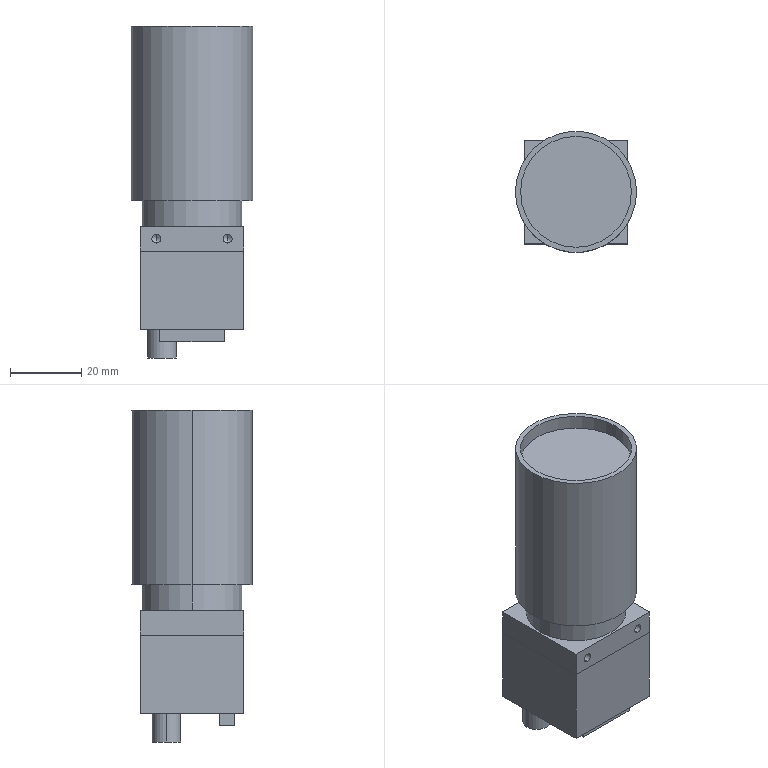Part | NX | features BREP 2 | 2 solids | 45 faces | box 34 x 34 x 93.2 mm | volume 70795 mm3 | plane 21 | cylinder 16 | cone 8 | commonest cylinder face diameters 2.5 x8 7.998 x2 28 x2 31.136 x2 34 x2
STEP:
#1=CARTESIAN_POINT('',(-12.39,7.192,-8.));
#2=VERTEX_POINT('',#1);
#3=CARTESIAN_POINT('',(-4.391,7.192,-8.));
#4=VERTEX_POINT('',#3);
#5=CARTESIAN_POINT('',(-8.39,7.192,-8.));
#6=DIRECTION('',(0.,0.,-1.));
#7=DIRECTION('',(-1.,0.,0.));
#8=AXIS2_PLACEMENT_3D('',#5,#6,#7);
#9=CIRCLE('',#8,3.999);
#10=EDGE_CURVE('',#2,#4,#9,.T.);
#11=ORIENTED_EDGE('',*,*,#10,.F.);
#12=CARTESIAN_POINT('',(-12.39,7.192,0.));
#13=VERTEX_POINT('',#12);
#14=CARTESIAN_POINT('',(-12.39,7.192,-8.));
#15=DIRECTION('',(0.,0.,1.));
#16=VECTOR('',#15,1000.);
#17=LINE('',#14,#16);
#18=EDGE_CURVE('',#13,#2,#17,.F.);
#19=ORIENTED_EDGE('',*,*,#18,.F.);
#20=CARTESIAN_POINT('',(-4.391,7.192,0.));
#21=VERTEX_POINT('',#20);
#22=CARTESIAN_POINT('',(-8.39,7.192,0.));
#23=DIRECTION('',(0.,0.,-1.));
#24=DIRECTION('',(-1.,0.,0.));
#25=AXIS2_PLACEMENT_3D('',#22,#23,#24);
#26=CIRCLE('',#25,3.999);
#27=EDGE_CURVE('',#13,#21,#26,.T.);
#28=ORIENTED_EDGE('',*,*,#27,.T.);
#29=CARTESIAN_POINT('',(-4.391,7.192,-8.));
#30=DIRECTION('',(0.,0.,1.));
#31=VECTOR('',#30,1000.);
#32=LINE('',#29,#31);
#33=EDGE_CURVE('',#21,#4,#32,.F.);
#34=ORIENTED_EDGE('',*,*,#33,.T.);
#35=EDGE_LOOP('',(#11,#19,#28,#34));
#36=FACE_BOUND('',#35,.T.);
#37=CARTESIAN_POINT('',(-8.39,7.192,-8.));
#38=DIRECTION('',(0.,0.,1.));
#39=DIRECTION('',(1.,0.,0.));
#40=AXIS2_PLACEMENT_3D('',#37,#38,#39);
#41=CYLINDRICAL_SURFACE('',#40,3.999);
#42=ADVANCED_FACE('',(#36),#41,.T.);
#43=CARTESIAN_POINT('',(14.5,-14.5,0.));
#44=VERTEX_POINT('',#43);
#45=CARTESIAN_POINT('',(14.5,14.5,0.));
#46=VERTEX_POINT('',#45);
#47=CARTESIAN_POINT('',(14.5,-14.5,0.));
#48=DIRECTION('',(0.,1.,0.));
#49=VECTOR('',#48,1000.);
#50=LINE('',#47,#49);
#51=EDGE_CURVE('',#44,#46,#50,.T.);
#52=ORIENTED_EDGE('',*,*,#51,.F.);
#53=CARTESIAN_POINT('',(-14.5,-14.5,0.));
#54=VERTEX_POINT('',#53);
#55=CARTESIAN_POINT('',(-14.5,-14.5,0.));
#56=DIRECTION('',(1.,0.,0.));
#57=VECTOR('',#56,1000.);
#58=LINE('',#55,#57);
#59=EDGE_CURVE('',#54,#44,#58,.T.);
#60=ORIENTED_EDGE('',*,*,#59,.F.);
#61=CARTESIAN_POINT('',(-14.5,14.5,0.));
#62=VERTEX_POINT('',#61);
#63=CARTESIAN_POINT('',(-14.5,-14.5,0.));
#64=DIRECTION('',(0.,-1.,0.));
#65=VECTOR('',#64,1000.);
#66=LINE('',#63,#65);
#67=EDGE_CURVE('',#62,#54,#66,.T.);
#68=ORIENTED_EDGE('',*,*,#67,.F.);
#69=CARTESIAN_POINT('',(-14.5,14.5,0.));
#70=DIRECTION('',(-1.,0.,0.));
#71=VECTOR('',#70,1000.);
#72=LINE('',#69,#71);
#73=EDGE_CURVE('',#46,#62,#72,.T.);
#74=ORIENTED_EDGE('',*,*,#73,.F.);
#75=EDGE_LOOP('',(#52,#60,#68,#74));
#76=FACE_BOUND('',#75,.T.);
#77=CARTESIAN_POINT('',(9.023,-12.03,0.));
#78=VERTEX_POINT('',#77);
#79=CARTESIAN_POINT('',(-9.023,-12.03,0.));
#80=VERTEX_POINT('',#79);
#81=CARTESIAN_POINT('',(-9.023,-12.03,0.));
#82=DIRECTION('',(-1.,0.,0.));
#83=VECTOR('',#82,1000.);
#84=LINE('',#81,#83);
#85=EDGE_CURVE('',#78,#80,#84,.T.);
#86=ORIENTED_EDGE('',*,*,#85,.F.);
#87=CARTESIAN_POINT('',(9.023,-7.6,0.));
#88=VERTEX_POINT('',#87);
#89=CARTESIAN_POINT('',(9.023,-12.03,0.));
#90=DIRECTION('',(0.,-1.,0.));
#91=VECTOR('',#90,1000.);
#92=LINE('',#89,#91);
#93=EDGE_CURVE('',#88,#78,#92,.T.);
#94=ORIENTED_EDGE('',*,*,#93,.F.);
#95=CARTESIAN_POINT('',(-9.023,-7.6,0.));
#96=VERTEX_POINT('',#95);
#97=CARTESIAN_POINT('',(-9.023,-7.6,0.));
#98=DIRECTION('',(1.,0.,0.));
#99=VECTOR('',#98,1000.);
#100=LINE('',#97,#99);
#101=EDGE_CURVE('',#96,#88,#100,.T.);
#102=ORIENTED_EDGE('',*,*,#101,.F.);
#103=CARTESIAN_POINT('',(-9.023,-12.03,0.));
#104=DIRECTION('',(0.,1.,0.));
#105=VECTOR('',#104,1000.);
#106=LINE('',#103,#105);
#107=EDGE_CURVE('',#80,#96,#106,.T.);
#108=ORIENTED_EDGE('',*,*,#107,.F.);
#109=EDGE_LOOP('',(#86,#94,#102,#108));
#110=FACE_BOUND('',#109,.T.);
#111=CARTESIAN_POINT('',(-8.39,7.192,0.));
#112=DIRECTION('',(0.,0.,-1.));
#113=DIRECTION('',(-1.,0.,0.));
#114=AXIS2_PLACEMENT_3D('',#111,#112,#113);
#115=CIRCLE('',#114,3.999);
#116=EDGE_CURVE('',#21,#13,#115,.T.);
#117=ORIENTED_EDGE('',*,*,#116,.F.);
#118=ORIENTED_EDGE('',*,*,#27,.F.);
#119=EDGE_LOOP('',(#117,#118));
#120=FACE_BOUND('',#119,.T.);
#121=CARTESIAN_POINT('',(0.,0.,0.));
#122=DIRECTION('',(0.,0.,-1.));
#123=DIRECTION('',(0.,-1.,0.));
#124=AXIS2_PLACEMENT_3D('',#121,#122,#123);
#125=PLANE('',#124);
#126=ADVANCED_FACE('',(#76,#110,#120),#125,.T.);
#127=ORIENTED_EDGE('',*,*,#51,.T.);
#128=CARTESIAN_POINT('',(14.5,14.5,22.));
#129=VERTEX_POINT('',#128);
#130=CARTESIAN_POINT('',(14.5,14.5,22.));
#131=DIRECTION('',(0.,0.,-1.));
#132=VECTOR('',#131,1000.);
#133=LINE('',#130,#132);
#134=EDGE_CURVE('',#129,#46,#133,.T.);
#135=ORIENTED_EDGE('',*,*,#134,.F.);
#136=CARTESIAN_POINT('',(14.5,-14.5,22.));
#137=VERTEX_POINT('',#136);
#138=CARTESIAN_POINT('',(14.5,-14.5,22.));
#139=DIRECTION('',(0.,1.,0.));
#140=VECTOR('',#139,1000.);
#141=LINE('',#138,#140);
#142=EDGE_CURVE('',#137,#129,#141,.T.);
#143=ORIENTED_EDGE('',*,*,#142,.F.);
#144=CARTESIAN_POINT('',(14.5,-14.5,22.));
#145=DIRECTION('',(0.,0.,-1.));
#146=VECTOR('',#145,1000.);
#147=LINE('',#144,#146);
#148=EDGE_CURVE('',#137,#44,#147,.T.);
#149=ORIENTED_EDGE('',*,*,#148,.T.);
#150=EDGE_LOOP('',(#127,#135,#143,#149));
#151=FACE_BOUND('',#150,.T.);
#152=CARTESIAN_POINT('',(14.5,-14.5,22.));
#153=DIRECTION('',(-1.,0.,0.));
#154=DIRECTION('',(0.,0.,1.));
#155=AXIS2_PLACEMENT_3D('',#152,#153,#154);
#156=PLANE('',#155);
#157=ADVANCED_FACE('',(#151),#156,.F.);
#158=ORIENTED_EDGE('',*,*,#73,.T.);
#159=CARTESIAN_POINT('',(-14.5,14.5,22.));
#160=VERTEX_POINT('',#159);
#161=CARTESIAN_POINT('',(-14.5,14.5,22.));
#162=DIRECTION('',(0.,0.,-1.));
#163=VECTOR('',#162,1000.);
#164=LINE('',#161,#163);
#165=EDGE_CURVE('',#160,#62,#164,.T.);
#166=ORIENTED_EDGE('',*,*,#165,.F.);
#167=CARTESIAN_POINT('',(-14.5,14.5,22.));
#168=DIRECTION('',(-1.,0.,0.));
#169=VECTOR('',#168,1000.);
#170=LINE('',#167,#169);
#171=EDGE_CURVE('',#129,#160,#170,.T.);
#172=ORIENTED_EDGE('',*,*,#171,.F.);
#173=ORIENTED_EDGE('',*,*,#134,.T.);
#174=EDGE_LOOP('',(#158,#166,#172,#173));
#175=FACE_BOUND('',#174,.T.);
#176=CARTESIAN_POINT('',(-14.5,14.5,22.));
#177=DIRECTION('',(0.,-1.,0.));
#178=DIRECTION('',(0.,0.,-1.));
#179=AXIS2_PLACEMENT_3D('',#176,#177,#178);
#180=PLANE('',#179);
#181=ADVANCED_FACE('',(#175),#180,.F.);
#182=ORIENTED_EDGE('',*,*,#67,.T.);
#183=CARTESIAN_POINT('',(-14.5,-14.5,22.));
#184=VERTEX_POINT('',#183);
#185=CARTESIAN_POINT('',(-14.5,-14.5,22.));
#186=DIRECTION('',(0.,0.,-1.));
#187=VECTOR('',#186,1000.);
#188=LINE('',#185,#187);
#189=EDGE_CURVE('',#184,#54,#188,.T.);
#190=ORIENTED_EDGE('',*,*,#189,.F.);
#191=CARTESIAN_POINT('',(-14.5,-14.5,22.));
#192=DIRECTION('',(0.,-1.,0.));
#193=VECTOR('',#192,1000.);
#194=LINE('',#191,#193);
#195=EDGE_CURVE('',#160,#184,#194,.T.);
#196=ORIENTED_EDGE('',*,*,#195,.F.);
#197=ORIENTED_EDGE('',*,*,#165,.T.);
#198=EDGE_LOOP('',(#182,#190,#196,#197));
#199=FACE_BOUND('',#198,.T.);
#200=CARTESIAN_POINT('',(-14.5,-14.5,22.));
#201=DIRECTION('',(1.,0.,0.));
#202=DIRECTION('',(0.,1.,0.));
#203=AXIS2_PLACEMENT_3D('',#200,#201,#202);
#204=PLANE('',#203);
#205=ADVANCED_FACE('',(#199),#204,.F.);
#206=ORIENTED_EDGE('',*,*,#59,.T.);
#207=ORIENTED_EDGE('',*,*,#148,.F.);
#208=CARTESIAN_POINT('',(-14.5,-14.5,22.));
#209=DIRECTION('',(1.,0.,0.));
#210=VECTOR('',#209,1000.);
#211=LINE('',#208,#210);
#212=EDGE_CURVE('',#184,#137,#211,.T.);
#213=ORIENTED_EDGE('',*,*,#212,.F.);
#214=ORIENTED_EDGE('',*,*,#189,.T.);
#215=EDGE_LOOP('',(#206,#207,#213,#214));
#216=FACE_BOUND('',#215,.T.);
#217=CARTESIAN_POINT('',(-14.5,-14.5,22.));
#218=DIRECTION('',(0.,1.,0.));
#219=DIRECTION('',(1.,0.,0.));
#220=AXIS2_PLACEMENT_3D('',#217,#218,#219);
#221=PLANE('',#220);
#222=ADVANCED_FACE('',(#216),#221,.F.);
#223=ORIENTED_EDGE('',*,*,#142,.T.);
#224=ORIENTED_EDGE('',*,*,#171,.T.);
#225=ORIENTED_EDGE('',*,*,#195,.T.);
#226=ORIENTED_EDGE('',*,*,#212,.T.);
#227=EDGE_LOOP('',(#223,#224,#225,#226));
#228=FACE_BOUND('',#227,.T.);
#229=CARTESIAN_POINT('',(0.,0.,22.));
#230=DIRECTION('',(0.,0.,-1.));
#231=DIRECTION('',(0.,-1.,0.));
#232=AXIS2_PLACEMENT_3D('',#229,#230,#231);
#233=PLANE('',#232);
#234=ADVANCED_FACE('',(#228),#233,.F.);
#235=ORIENTED_EDGE('',*,*,#93,.T.);
#236=CARTESIAN_POINT('',(9.023,-12.03,-3.5));
#237=VERTEX_POINT('',#236);
#238=CARTESIAN_POINT('',(9.023,-12.03,-3.5));
#239=DIRECTION('',(0.,0.,1.));
#240=VECTOR('',#239,1000.);
#241=LINE('',#238,#240);
#242=EDGE_CURVE('',#237,#78,#241,.T.);
#243=ORIENTED_EDGE('',*,*,#242,.F.);
#244=CARTESIAN_POINT('',(9.023,-7.6,-3.5));
#245=VERTEX_POINT('',#244);
#246=CARTESIAN_POINT('',(9.023,-12.03,-3.5));
#247=DIRECTION('',(0.,-1.,0.));
#248=VECTOR('',#247,1000.);
#249=LINE('',#246,#248);
#250=EDGE_CURVE('',#245,#237,#249,.T.);
#251=ORIENTED_EDGE('',*,*,#250,.F.);
#252=CARTESIAN_POINT('',(9.023,-7.6,-3.5));
#253=DIRECTION('',(0.,0.,1.));
#254=VECTOR('',#253,1000.);
#255=LINE('',#252,#254);
#256=EDGE_CURVE('',#245,#88,#255,.T.);
#257=ORIENTED_EDGE('',*,*,#256,.T.);
#258=EDGE_LOOP('',(#235,#243,#251,#257));
#259=FACE_BOUND('',#258,.T.);
#260=CARTESIAN_POINT('',(9.023,-12.03,-3.5));
#261=DIRECTION('',(-1.,0.,0.));
#262=DIRECTION('',(0.,0.,1.));
#263=AXIS2_PLACEMENT_3D('',#260,#261,#262);
#264=PLANE('',#263);
#265=ADVANCED_FACE('',(#259),#264,.F.);
#266=ORIENTED_EDGE('',*,*,#85,.T.);
#267=CARTESIAN_POINT('',(-9.023,-12.03,-3.5));
#268=VERTEX_POINT('',#267);
#269=CARTESIAN_POINT('',(-9.023,-12.03,-3.5));
#270=DIRECTION('',(0.,0.,1.));
#271=VECTOR('',#270,1000.);
#272=LINE('',#269,#271);
#273=EDGE_CURVE('',#268,#80,#272,.T.);
#274=ORIENTED_EDGE('',*,*,#273,.F.);
#275=CARTESIAN_POINT('',(-9.023,-12.03,-3.5));
#276=DIRECTION('',(-1.,0.,0.));
#277=VECTOR('',#276,1000.);
#278=LINE('',#275,#277);
#279=EDGE_CURVE('',#237,#268,#278,.T.);
#280=ORIENTED_EDGE('',*,*,#279,.F.);
#281=ORIENTED_EDGE('',*,*,#242,.T.);
#282=EDGE_LOOP('',(#266,#274,#280,#281));
#283=FACE_BOUND('',#282,.T.);
#284=CARTESIAN_POINT('',(-9.023,-12.03,-3.5));
#285=DIRECTION('',(0.,1.,0.));
#286=DIRECTION('',(1.,0.,0.));
#287=AXIS2_PLACEMENT_3D('',#284,#285,#286);
#288=PLANE('',#287);
#289=ADVANCED_FACE('',(#283),#288,.F.);
#290=ORIENTED_EDGE('',*,*,#107,.T.);
#291=CARTESIAN_POINT('',(-9.023,-7.6,-3.5));
#292=VERTEX_POINT('',#291);
#293=CARTESIAN_POINT('',(-9.023,-7.6,-3.5));
#294=DIRECTION('',(0.,0.,1.));
#295=VECTOR('',#294,1000.);
#296=LINE('',#293,#295);
#297=EDGE_CURVE('',#292,#96,#296,.T.);
#298=ORIENTED_EDGE('',*,*,#297,.F.);
#299=CARTESIAN_POINT('',(-9.023,-12.03,-3.5));
#300=DIRECTION('',(0.,1.,0.));
#301=VECTOR('',#300,1000.);
#302=LINE('',#299,#301);
#303=EDGE_CURVE('',#268,#292,#302,.T.);
#304=ORIENTED_EDGE('',*,*,#303,.F.);
#305=ORIENTED_EDGE('',*,*,#273,.T.);
#306=EDGE_LOOP('',(#290,#298,#304,#305));
#307=FACE_BOUND('',#306,.T.);
#308=CARTESIAN_POINT('',(-9.023,-12.03,-3.5));
#309=DIRECTION('',(1.,0.,0.));
#310=DIRECTION('',(0.,1.,0.));
#311=AXIS2_PLACEMENT_3D('',#308,#309,#310);
#312=PLANE('',#311);
#313=ADVANCED_FACE('',(#307),#312,.F.);
#314=ORIENTED_EDGE('',*,*,#101,.T.);
#315=ORIENTED_EDGE('',*,*,#256,.F.);
#316=CARTESIAN_POINT('',(-9.023,-7.6,-3.5));
#317=DIRECTION('',(1.,0.,0.));
#318=VECTOR('',#317,1000.);
#319=LINE('',#316,#318);
#320=EDGE_CURVE('',#292,#245,#319,.T.);
#321=ORIENTED_EDGE('',*,*,#320,.F.);
#322=ORIENTED_EDGE('',*,*,#297,.T.);
#323=EDGE_LOOP('',(#314,#315,#321,#322));
#324=FACE_BOUND('',#323,.T.);
#325=CARTESIAN_POINT('',(-9.023,-7.6,-3.5));
#326=DIRECTION('',(0.,-1.,0.));
#327=DIRECTION('',(0.,0.,-1.));
#328=AXIS2_PLACEMENT_3D('',#325,#326,#327);
#329=PLANE('',#328);
#330=ADVANCED_FACE('',(#324),#329,.F.);
#331=ORIENTED_EDGE('',*,*,#250,.T.);
#332=ORIENTED_EDGE('',*,*,#279,.T.);
#333=ORIENTED_EDGE('',*,*,#303,.T.);
#334=ORIENTED_EDGE('',*,*,#320,.T.);
#335=EDGE_LOOP('',(#331,#332,#333,#334));
#336=FACE_BOUND('',#335,.T.);
#337=CARTESIAN_POINT('',(0.,0.,-3.5));
#338=DIRECTION('',(0.,0.,-1.));
#339=DIRECTION('',(0.,-1.,0.));
#340=AXIS2_PLACEMENT_3D('',#337,#338,#339);
#341=PLANE('',#340);
#342=ADVANCED_FACE('',(#336),#341,.T.);
#343=ORIENTED_EDGE('',*,*,#18,.T.);
#344=CARTESIAN_POINT('',(-8.39,7.192,-8.));
#345=DIRECTION('',(0.,0.,-1.));
#346=DIRECTION('',(-1.,0.,0.));
#347=AXIS2_PLACEMENT_3D('',#344,#345,#346);
#348=CIRCLE('',#347,3.999);
#349=EDGE_CURVE('',#4,#2,#348,.T.);
#350=ORIENTED_EDGE('',*,*,#349,.F.);
#351=ORIENTED_EDGE('',*,*,#33,.F.);
#352=ORIENTED_EDGE('',*,*,#116,.T.);
#353=EDGE_LOOP('',(#343,#350,#351,#352));
#354=FACE_BOUND('',#353,.T.);
#355=CARTESIAN_POINT('',(-8.39,7.192,-8.));
#356=DIRECTION('',(0.,0.,1.));
#357=DIRECTION('',(1.,0.,0.));
#358=AXIS2_PLACEMENT_3D('',#355,#356,#357);
#359=CYLINDRICAL_SURFACE('',#358,3.999);
#360=ADVANCED_FACE('',(#354),#359,.T.);
#361=ORIENTED_EDGE('',*,*,#349,.T.);
#362=ORIENTED_EDGE('',*,*,#10,.T.);
#363=EDGE_LOOP('',(#361,#362));
#364=FACE_BOUND('',#363,.T.);
#365=CARTESIAN_POINT('',(-8.39,7.192,-8.));
#366=DIRECTION('',(0.,0.,-1.));
#367=DIRECTION('',(0.,-1.,0.));
#368=AXIS2_PLACEMENT_3D('',#365,#366,#367);
#369=PLANE('',#368);
#370=ADVANCED_FACE('',(#364),#369,.T.);
#371=CLOSED_SHELL('',(#42,#126,#157,#181,#205,#222,#234,#265,#289,#313,#330,#342,#360,#370));
#372=MANIFOLD_SOLID_BREP('',#371);
#373=CARTESIAN_POINT('',(-15.568,0.,81.2));
#374=VERTEX_POINT('',#373);
#375=CARTESIAN_POINT('',(15.568,0.,81.2));
#376=VERTEX_POINT('',#375);
#377=CARTESIAN_POINT('',(0.,0.,81.2));
#378=DIRECTION('',(0.,0.,1.));
#379=DIRECTION('',(1.,0.,0.));
#380=AXIS2_PLACEMENT_3D('',#377,#378,#379);
#381=CIRCLE('',#380,15.568);
#382=EDGE_CURVE('',#374,#376,#381,.T.);
#383=ORIENTED_EDGE('',*,*,#382,.F.);
#384=CARTESIAN_POINT('',(-15.568,0.,85.2));
#385=VERTEX_POINT('',#384);
#386=CARTESIAN_POINT('',(-15.568,0.,81.2));
#387=DIRECTION('',(0.,0.,1.));
#388=VECTOR('',#387,1000.);
#389=LINE('',#386,#388);
#390=EDGE_CURVE('',#385,#374,#389,.F.);
#391=ORIENTED_EDGE('',*,*,#390,.F.);
#392=CARTESIAN_POINT('',(15.568,0.,85.2));
#393=VERTEX_POINT('',#392);
#394=CARTESIAN_POINT('',(0.,0.,85.2));
#395=DIRECTION('',(0.,0.,1.));
#396=DIRECTION('',(1.,0.,0.));
#397=AXIS2_PLACEMENT_3D('',#394,#395,#396);
#398=CIRCLE('',#397,15.568);
#399=EDGE_CURVE('',#385,#393,#398,.T.);
#400=ORIENTED_EDGE('',*,*,#399,.T.);
#401=CARTESIAN_POINT('',(15.568,0.,81.2));
#402=DIRECTION('',(0.,0.,1.));
#403=VECTOR('',#402,1000.);
#404=LINE('',#401,#403);
#405=EDGE_CURVE('',#393,#376,#404,.F.);
#406=ORIENTED_EDGE('',*,*,#405,.T.);
#407=EDGE_LOOP('',(#383,#391,#400,#406));
#408=FACE_BOUND('',#407,.T.);
#409=CARTESIAN_POINT('',(0.,0.,81.2));
#410=DIRECTION('',(0.,0.,1.));
#411=DIRECTION('',(1.,0.,0.));
#412=AXIS2_PLACEMENT_3D('',#409,#410,#411);
#413=CYLINDRICAL_SURFACE('',#412,15.568);
#414=ADVANCED_FACE('',(#408),#413,.F.);
#415=CARTESIAN_POINT('',(17.,0.,85.2));
#416=VERTEX_POINT('',#415);
#417=CARTESIAN_POINT('',(-17.,0.,85.2));
#418=VERTEX_POINT('',#417);
#419=CARTESIAN_POINT('',(0.,0.,85.2));
#420=DIRECTION('',(0.,0.,1.));
#421=DIRECTION('',(1.,0.,0.));
#422=AXIS2_PLACEMENT_3D('',#419,#420,#421);
#423=CIRCLE('',#422,17.);
#424=EDGE_CURVE('',#416,#418,#423,.T.);
#425=ORIENTED_EDGE('',*,*,#424,.F.);
#426=CARTESIAN_POINT('',(17.,0.,36.2));
#427=VERTEX_POINT('',#426);
#428=CARTESIAN_POINT('',(17.,0.,85.2));
#429=DIRECTION('',(0.,0.,-1.));
#430=VECTOR('',#429,1000.);
#431=LINE('',#428,#430);
#432=EDGE_CURVE('',#416,#427,#431,.T.);
#433=ORIENTED_EDGE('',*,*,#432,.T.);
#434=CARTESIAN_POINT('',(-17.,0.,36.2));
#435=VERTEX_POINT('',#434);
#436=CARTESIAN_POINT('',(0.,0.,36.2));
#437=DIRECTION('',(0.,0.,1.));
#438=DIRECTION('',(1.,0.,0.));
#439=AXIS2_PLACEMENT_3D('',#436,#437,#438);
#440=CIRCLE('',#439,17.);
#441=EDGE_CURVE('',#427,#435,#440,.T.);
#442=ORIENTED_EDGE('',*,*,#441,.T.);
#443=CARTESIAN_POINT('',(-17.,0.,85.2));
#444=DIRECTION('',(0.,0.,-1.));
#445=VECTOR('',#444,1000.);
#446=LINE('',#443,#445);
#447=EDGE_CURVE('',#418,#435,#446,.T.);
#448=ORIENTED_EDGE('',*,*,#447,.F.);
#449=EDGE_LOOP('',(#425,#433,#442,#448));
#450=FACE_BOUND('',#449,.T.);
#451=CARTESIAN_POINT('',(0.,0.,85.2));
#452=DIRECTION('',(0.,0.,-1.));
#453=DIRECTION('',(-1.,0.,0.));
#454=AXIS2_PLACEMENT_3D('',#451,#452,#453);
#455=CYLINDRICAL_SURFACE('',#454,17.);
#456=ADVANCED_FACE('',(#450),#455,.T.);
#457=CARTESIAN_POINT('',(14.,0.,36.2));
#458=VERTEX_POINT('',#457);
#459=CARTESIAN_POINT('',(-14.,0.,36.2));
#460=VERTEX_POINT('',#459);
#461=CARTESIAN_POINT('',(0.,0.,36.2));
#462=DIRECTION('',(0.,0.,1.));
#463=DIRECTION('',(1.,0.,0.));
#464=AXIS2_PLACEMENT_3D('',#461,#462,#463);
#465=CIRCLE('',#464,14.);
#466=EDGE_CURVE('',#458,#460,#465,.T.);
#467=ORIENTED_EDGE('',*,*,#466,.F.);
#468=CARTESIAN_POINT('',(14.,0.,29.));
#469=VERTEX_POINT('',#468);
#470=CARTESIAN_POINT('',(14.,0.,36.2));
#471=DIRECTION('',(0.,0.,-1.));
#472=VECTOR('',#471,1000.);
#473=LINE('',#470,#472);
#474=EDGE_CURVE('',#458,#469,#473,.T.);
#475=ORIENTED_EDGE('',*,*,#474,.T.);
#476=CARTESIAN_POINT('',(-14.,0.,29.));
#477=VERTEX_POINT('',#476);
#478=CARTESIAN_POINT('',(0.,0.,29.));
#479=DIRECTION('',(0.,0.,1.));
#480=DIRECTION('',(1.,0.,0.));
#481=AXIS2_PLACEMENT_3D('',#478,#479,#480);
#482=CIRCLE('',#481,14.);
#483=EDGE_CURVE('',#469,#477,#482,.T.);
#484=ORIENTED_EDGE('',*,*,#483,.T.);
#485=CARTESIAN_POINT('',(-14.,0.,36.2));
#486=DIRECTION('',(0.,0.,-1.));
#487=VECTOR('',#486,1000.);
#488=LINE('',#485,#487);
#489=EDGE_CURVE('',#460,#477,#488,.T.);
#490=ORIENTED_EDGE('',*,*,#489,.F.);
#491=EDGE_LOOP('',(#467,#475,#484,#490));
#492=FACE_BOUND('',#491,.T.);
#493=CARTESIAN_POINT('',(0.,0.,36.2));
#494=DIRECTION('',(0.,0.,-1.));
#495=DIRECTION('',(-1.,0.,0.));
#496=AXIS2_PLACEMENT_3D('',#493,#494,#495);
#497=CYLINDRICAL_SURFACE('',#496,14.);
#498=ADVANCED_FACE('',(#492),#497,.T.);
#499=CARTESIAN_POINT('',(10.,-7.,26.75));
#500=VERTEX_POINT('',#499);
#501=CARTESIAN_POINT('',(10.,-7.,24.25));
#502=VERTEX_POINT('',#501);
#503=CARTESIAN_POINT('',(10.,-7.,25.5));
#504=DIRECTION('',(0.,-1.,0.));
#505=DIRECTION('',(0.,0.,-1.));
#506=AXIS2_PLACEMENT_3D('',#503,#504,#505);
#507=CIRCLE('',#506,1.25);
#508=EDGE_CURVE('',#500,#502,#507,.T.);
#509=ORIENTED_EDGE('',*,*,#508,.F.);
#510=CARTESIAN_POINT('',(10.,-14.5,26.75));
#511=VERTEX_POINT('',#510);
#512=CARTESIAN_POINT('',(10.,-14.5,26.75));
#513=DIRECTION('',(0.,-1.,0.));
#514=VECTOR('',#513,1000.);
#515=LINE('',#512,#514);
#516=EDGE_CURVE('',#500,#511,#515,.T.);
#517=ORIENTED_EDGE('',*,*,#516,.T.);
#518=CARTESIAN_POINT('',(10.,-14.5,24.25));
#519=VERTEX_POINT('',#518);
#520=CARTESIAN_POINT('',(10.,-14.5,25.5));
#521=DIRECTION('',(0.,-1.,0.));
#522=DIRECTION('',(0.,0.,-1.));
#523=AXIS2_PLACEMENT_3D('',#520,#521,#522);
#524=CIRCLE('',#523,1.25);
#525=EDGE_CURVE('',#511,#519,#524,.T.);
#526=ORIENTED_EDGE('',*,*,#525,.T.);
#527=CARTESIAN_POINT('',(10.,-14.5,24.25));
#528=DIRECTION('',(0.,-1.,0.));
#529=VECTOR('',#528,1000.);
#530=LINE('',#527,#529);
#531=EDGE_CURVE('',#502,#519,#530,.T.);
#532=ORIENTED_EDGE('',*,*,#531,.F.);
#533=EDGE_LOOP('',(#509,#517,#526,#532));
#534=FACE_BOUND('',#533,.T.);
#535=CARTESIAN_POINT('',(10.,-14.5,25.5));
#536=DIRECTION('',(0.,-1.,0.));
#537=DIRECTION('',(0.,0.,-1.));
#538=AXIS2_PLACEMENT_3D('',#535,#536,#537);
#539=CYLINDRICAL_SURFACE('',#538,1.25);
#540=ADVANCED_FACE('',(#534),#539,.F.);
#541=CARTESIAN_POINT('',(10.,-6.249,25.5));
#542=VERTEX_POINT('',#541);
#543=CARTESIAN_POINT('',(10.,-7.,24.25));
#544=DIRECTION('',(0.,-0.515,-0.8572));
#545=VECTOR('',#544,1000.);
#546=LINE('',#543,#545);
#547=EDGE_CURVE('',#542,#502,#546,.T.);
#548=ORIENTED_EDGE('',*,*,#547,.F.);
#549=CARTESIAN_POINT('',(10.,-7.,26.75));
#550=DIRECTION('',(0.,-0.515,0.8572));
#551=VECTOR('',#550,1000.);
#552=LINE('',#549,#551);
#553=EDGE_CURVE('',#542,#500,#552,.T.);
#554=ORIENTED_EDGE('',*,*,#553,.T.);
#555=ORIENTED_EDGE('',*,*,#508,.T.);
#556=EDGE_LOOP('',(#548,#554,#555));
#557=FACE_BOUND('',#556,.T.);
#558=CARTESIAN_POINT('',(10.,-7.,25.5));
#559=DIRECTION('',(0.,-1.,0.));
#560=DIRECTION('',(0.,0.,-1.));
#561=AXIS2_PLACEMENT_3D('',#558,#559,#560);
#562=CONICAL_SURFACE('',#561,1.25,1.03);
#563=ADVANCED_FACE('',(#557),#562,.F.);
#564=CARTESIAN_POINT('',(-10.,-7.,26.75));
#565=VERTEX_POINT('',#564);
#566=CARTESIAN_POINT('',(-10.,-7.,24.25));
#567=VERTEX_POINT('',#566);
#568=CARTESIAN_POINT('',(-10.,-7.,25.5));
#569=DIRECTION('',(0.,-1.,0.));
#570=DIRECTION('',(0.,0.,-1.));
#571=AXIS2_PLACEMENT_3D('',#568,#569,#570);
#572=CIRCLE('',#571,1.25);
#573=EDGE_CURVE('',#565,#567,#572,.T.);
#574=ORIENTED_EDGE('',*,*,#573,.F.);
#575=CARTESIAN_POINT('',(-10.,-14.5,26.75));
#576=VERTEX_POINT('',#575);
#577=CARTESIAN_POINT('',(-10.,-14.5,26.75));
#578=DIRECTION('',(0.,-1.,0.));
#579=VECTOR('',#578,1000.);
#580=LINE('',#577,#579);
#581=EDGE_CURVE('',#565,#576,#580,.T.);
#582=ORIENTED_EDGE('',*,*,#581,.T.);
#583=CARTESIAN_POINT('',(-10.,-14.5,24.25));
#584=VERTEX_POINT('',#583);
#585=CARTESIAN_POINT('',(-10.,-14.5,25.5));
#586=DIRECTION('',(0.,-1.,0.));
#587=DIRECTION('',(0.,0.,-1.));
#588=AXIS2_PLACEMENT_3D('',#585,#586,#587);
#589=CIRCLE('',#588,1.25);
#590=EDGE_CURVE('',#576,#584,#589,.T.);
#591=ORIENTED_EDGE('',*,*,#590,.T.);
#592=CARTESIAN_POINT('',(-10.,-14.5,24.25));
#593=DIRECTION('',(0.,-1.,0.));
#594=VECTOR('',#593,1000.);
#595=LINE('',#592,#594);
#596=EDGE_CURVE('',#567,#584,#595,.T.);
#597=ORIENTED_EDGE('',*,*,#596,.F.);
#598=EDGE_LOOP('',(#574,#582,#591,#597));
#599=FACE_BOUND('',#598,.T.);
#600=CARTESIAN_POINT('',(-10.,-14.5,25.5));
#601=DIRECTION('',(0.,-1.,0.));
#602=DIRECTION('',(0.,0.,-1.));
#603=AXIS2_PLACEMENT_3D('',#600,#601,#602);
#604=CYLINDRICAL_SURFACE('',#603,1.25);
#605=ADVANCED_FACE('',(#599),#604,.F.);
#606=CARTESIAN_POINT('',(-10.,-6.249,25.5));
#607=VERTEX_POINT('',#606);
#608=CARTESIAN_POINT('',(-10.,-7.,24.25));
#609=DIRECTION('',(0.,-0.515,-0.8572));
#610=VECTOR('',#609,1000.);
#611=LINE('',#608,#610);
#612=EDGE_CURVE('',#607,#567,#611,.T.);
#613=ORIENTED_EDGE('',*,*,#612,.F.);
#614=CARTESIAN_POINT('',(-10.,-7.,26.75));
#615=DIRECTION('',(0.,-0.515,0.8572));
#616=VECTOR('',#615,1000.);
#617=LINE('',#614,#616);
#618=EDGE_CURVE('',#607,#565,#617,.T.);
#619=ORIENTED_EDGE('',*,*,#618,.T.);
#620=ORIENTED_EDGE('',*,*,#573,.T.);
#621=EDGE_LOOP('',(#613,#619,#620));
#622=FACE_BOUND('',#621,.T.);
#623=CARTESIAN_POINT('',(-10.,-7.,25.5));
#624=DIRECTION('',(0.,-1.,0.));
#625=DIRECTION('',(0.,0.,-1.));
#626=AXIS2_PLACEMENT_3D('',#623,#624,#625);
#627=CONICAL_SURFACE('',#626,1.25,1.03);
#628=ADVANCED_FACE('',(#622),#627,.F.);
#629=CARTESIAN_POINT('',(10.,7.,24.25));
#630=VERTEX_POINT('',#629);
#631=CARTESIAN_POINT('',(10.,7.,26.75));
#632=VERTEX_POINT('',#631);
#633=CARTESIAN_POINT('',(10.,7.,25.5));
#634=DIRECTION('',(0.,1.,0.));
#635=DIRECTION('',(0.,0.,1.));
#636=AXIS2_PLACEMENT_3D('',#633,#634,#635);
#637=CIRCLE('',#636,1.25);
#638=EDGE_CURVE('',#630,#632,#637,.T.);
#639=ORIENTED_EDGE('',*,*,#638,.F.);
#640=CARTESIAN_POINT('',(10.,14.5,24.25));
#641=VERTEX_POINT('',#640);
#642=CARTESIAN_POINT('',(10.,14.5,24.25));
#643=DIRECTION('',(0.,1.,0.));
#644=VECTOR('',#643,1000.);
#645=LINE('',#642,#644);
#646=EDGE_CURVE('',#641,#630,#645,.F.);
#647=ORIENTED_EDGE('',*,*,#646,.F.);
#648=CARTESIAN_POINT('',(10.,14.5,26.75));
#649=VERTEX_POINT('',#648);
#650=CARTESIAN_POINT('',(10.,14.5,25.5));
#651=DIRECTION('',(0.,1.,0.));
#652=DIRECTION('',(0.,0.,1.));
#653=AXIS2_PLACEMENT_3D('',#650,#651,#652);
#654=CIRCLE('',#653,1.25);
#655=EDGE_CURVE('',#641,#649,#654,.T.);
#656=ORIENTED_EDGE('',*,*,#655,.T.);
#657=CARTESIAN_POINT('',(10.,14.5,26.75));
#658=DIRECTION('',(0.,1.,0.));
#659=VECTOR('',#658,1000.);
#660=LINE('',#657,#659);
#661=EDGE_CURVE('',#649,#632,#660,.F.);
#662=ORIENTED_EDGE('',*,*,#661,.T.);
#663=EDGE_LOOP('',(#639,#647,#656,#662));
#664=FACE_BOUND('',#663,.T.);
#665=CARTESIAN_POINT('',(10.,14.5,25.5));
#666=DIRECTION('',(0.,1.,0.));
#667=DIRECTION('',(0.,0.,1.));
#668=AXIS2_PLACEMENT_3D('',#665,#666,#667);
#669=CYLINDRICAL_SURFACE('',#668,1.25);
#670=ADVANCED_FACE('',(#664),#669,.F.);
#671=CARTESIAN_POINT('',(10.,6.249,25.5));
#672=VERTEX_POINT('',#671);
#673=CARTESIAN_POINT('',(10.,7.,26.75));
#674=DIRECTION('',(0.,0.515,0.8572));
#675=VECTOR('',#674,1000.);
#676=LINE('',#673,#675);
#677=EDGE_CURVE('',#632,#672,#676,.F.);
#678=ORIENTED_EDGE('',*,*,#677,.T.);
#679=CARTESIAN_POINT('',(10.,7.,24.25));
#680=DIRECTION('',(0.,0.515,-0.8572));
#681=VECTOR('',#680,1000.);
#682=LINE('',#679,#681);
#683=EDGE_CURVE('',#630,#672,#682,.F.);
#684=ORIENTED_EDGE('',*,*,#683,.F.);
#685=ORIENTED_EDGE('',*,*,#638,.T.);
#686=EDGE_LOOP('',(#678,#684,#685));
#687=FACE_BOUND('',#686,.T.);
#688=CARTESIAN_POINT('',(10.,7.,25.5));
#689=DIRECTION('',(0.,1.,0.));
#690=DIRECTION('',(0.,0.,1.));
#691=AXIS2_PLACEMENT_3D('',#688,#689,#690);
#692=CONICAL_SURFACE('',#691,1.25,1.03);
#693=ADVANCED_FACE('',(#687),#692,.F.);
#694=CARTESIAN_POINT('',(-10.,7.,24.25));
#695=VERTEX_POINT('',#694);
#696=CARTESIAN_POINT('',(-10.,7.,26.75));
#697=VERTEX_POINT('',#696);
#698=CARTESIAN_POINT('',(-10.,7.,25.5));
#699=DIRECTION('',(0.,1.,0.));
#700=DIRECTION('',(0.,0.,1.));
#701=AXIS2_PLACEMENT_3D('',#698,#699,#700);
#702=CIRCLE('',#701,1.25);
#703=EDGE_CURVE('',#695,#697,#702,.T.);
#704=ORIENTED_EDGE('',*,*,#703,.F.);
#705=CARTESIAN_POINT('',(-10.,14.5,24.25));
#706=VERTEX_POINT('',#705);
#707=CARTESIAN_POINT('',(-10.,14.5,24.25));
#708=DIRECTION('',(0.,1.,0.));
#709=VECTOR('',#708,1000.);
#710=LINE('',#707,#709);
#711=EDGE_CURVE('',#706,#695,#710,.F.);
#712=ORIENTED_EDGE('',*,*,#711,.F.);
#713=CARTESIAN_POINT('',(-10.,14.5,26.75));
#714=VERTEX_POINT('',#713);
#715=CARTESIAN_POINT('',(-10.,14.5,25.5));
#716=DIRECTION('',(0.,1.,0.));
#717=DIRECTION('',(0.,0.,1.));
#718=AXIS2_PLACEMENT_3D('',#715,#716,#717);
#719=CIRCLE('',#718,1.25);
#720=EDGE_CURVE('',#706,#714,#719,.T.);
#721=ORIENTED_EDGE('',*,*,#720,.T.);
#722=CARTESIAN_POINT('',(-10.,14.5,26.75));
#723=DIRECTION('',(0.,1.,0.));
#724=VECTOR('',#723,1000.);
#725=LINE('',#722,#724);
#726=EDGE_CURVE('',#714,#697,#725,.F.);
#727=ORIENTED_EDGE('',*,*,#726,.T.);
#728=EDGE_LOOP('',(#704,#712,#721,#727));
#729=FACE_BOUND('',#728,.T.);
#730=CARTESIAN_POINT('',(-10.,14.5,25.5));
#731=DIRECTION('',(0.,1.,0.));
#732=DIRECTION('',(0.,0.,1.));
#733=AXIS2_PLACEMENT_3D('',#730,#731,#732);
#734=CYLINDRICAL_SURFACE('',#733,1.25);
#735=ADVANCED_FACE('',(#729),#734,.F.);
#736=CARTESIAN_POINT('',(-10.,6.249,25.5));
#737=VERTEX_POINT('',#736);
#738=CARTESIAN_POINT('',(-10.,7.,26.75));
#739=DIRECTION('',(0.,0.515,0.8572));
#740=VECTOR('',#739,1000.);
#741=LINE('',#738,#740);
#742=EDGE_CURVE('',#697,#737,#741,.F.);
#743=ORIENTED_EDGE('',*,*,#742,.T.);
#744=CARTESIAN_POINT('',(-10.,7.,24.25));
#745=DIRECTION('',(0.,0.515,-0.8572));
#746=VECTOR('',#745,1000.);
#747=LINE('',#744,#746);
#748=EDGE_CURVE('',#695,#737,#747,.F.);
#749=ORIENTED_EDGE('',*,*,#748,.F.);
#750=ORIENTED_EDGE('',*,*,#703,.T.);
#751=EDGE_LOOP('',(#743,#749,#750));
#752=FACE_BOUND('',#751,.T.);
#753=CARTESIAN_POINT('',(-10.,7.,25.5));
#754=DIRECTION('',(0.,1.,0.));
#755=DIRECTION('',(0.,0.,1.));
#756=AXIS2_PLACEMENT_3D('',#753,#754,#755);
#757=CONICAL_SURFACE('',#756,1.25,1.03);
#758=ADVANCED_FACE('',(#752),#757,.F.);
#759=CARTESIAN_POINT('',(-14.5,-14.5,29.));
#760=VERTEX_POINT('',#759);
#761=CARTESIAN_POINT('',(14.5,-14.5,29.));
#762=VERTEX_POINT('',#761);
#763=CARTESIAN_POINT('',(-14.5,-14.5,29.));
#764=DIRECTION('',(1.,0.,0.));
#765=VECTOR('',#764,1000.);
#766=LINE('',#763,#765);
#767=EDGE_CURVE('',#760,#762,#766,.T.);
#768=ORIENTED_EDGE('',*,*,#767,.T.);
#769=CARTESIAN_POINT('',(14.5,14.5,29.));
#770=VERTEX_POINT('',#769);
#771=CARTESIAN_POINT('',(14.5,-14.5,29.));
#772=DIRECTION('',(0.,1.,0.));
#773=VECTOR('',#772,1000.);
#774=LINE('',#771,#773);
#775=EDGE_CURVE('',#762,#770,#774,.T.);
#776=ORIENTED_EDGE('',*,*,#775,.T.);
#777=CARTESIAN_POINT('',(-14.5,14.5,29.));
#778=VERTEX_POINT('',#777);
#779=CARTESIAN_POINT('',(14.5,14.5,29.));
#780=DIRECTION('',(-1.,0.,0.));
#781=VECTOR('',#780,1000.);
#782=LINE('',#779,#781);
#783=EDGE_CURVE('',#770,#778,#782,.T.);
#784=ORIENTED_EDGE('',*,*,#783,.T.);
#785=CARTESIAN_POINT('',(-14.5,14.5,29.));
#786=DIRECTION('',(0.,-1.,0.));
#787=VECTOR('',#786,1000.);
#788=LINE('',#785,#787);
#789=EDGE_CURVE('',#778,#760,#788,.T.);
#790=ORIENTED_EDGE('',*,*,#789,.T.);
#791=EDGE_LOOP('',(#768,#776,#784,#790));
#792=FACE_BOUND('',#791,.T.);
#793=CARTESIAN_POINT('',(0.,0.,29.));
#794=DIRECTION('',(0.,0.,1.));
#795=DIRECTION('',(1.,0.,0.));
#796=AXIS2_PLACEMENT_3D('',#793,#794,#795);
#797=CIRCLE('',#796,14.);
#798=EDGE_CURVE('',#477,#469,#797,.T.);
#799=ORIENTED_EDGE('',*,*,#798,.F.);
#800=ORIENTED_EDGE('',*,*,#483,.F.);
#801=EDGE_LOOP('',(#799,#800));
#802=FACE_BOUND('',#801,.T.);
#803=CARTESIAN_POINT('',(0.,0.,29.));
#804=DIRECTION('',(0.,0.,1.));
#805=DIRECTION('',(1.,0.,0.));
#806=AXIS2_PLACEMENT_3D('',#803,#804,#805);
#807=PLANE('',#806);
#808=ADVANCED_FACE('',(#792,#802),#807,.T.);
#809=CARTESIAN_POINT('',(-14.5,-14.5,22.));
#810=VERTEX_POINT('',#809);
#811=CARTESIAN_POINT('',(14.5,-14.5,22.));
#812=VERTEX_POINT('',#811);
#813=CARTESIAN_POINT('',(-14.5,-14.5,22.));
#814=DIRECTION('',(1.,0.,0.));
#815=VECTOR('',#814,1000.);
#816=LINE('',#813,#815);
#817=EDGE_CURVE('',#810,#812,#816,.T.);
#818=ORIENTED_EDGE('',*,*,#817,.T.);
#819=CARTESIAN_POINT('',(14.5,-14.5,29.));
#820=DIRECTION('',(0.,0.,-1.));
#821=VECTOR('',#820,1000.);
#822=LINE('',#819,#821);
#823=EDGE_CURVE('',#762,#812,#822,.T.);
#824=ORIENTED_EDGE('',*,*,#823,.F.);
#825=ORIENTED_EDGE('',*,*,#767,.F.);
#826=CARTESIAN_POINT('',(-14.5,-14.5,29.));
#827=DIRECTION('',(0.,0.,-1.));
#828=VECTOR('',#827,1000.);
#829=LINE('',#826,#828);
#830=EDGE_CURVE('',#760,#810,#829,.T.);
#831=ORIENTED_EDGE('',*,*,#830,.T.);
#832=EDGE_LOOP('',(#818,#824,#825,#831));
#833=FACE_BOUND('',#832,.T.);
#834=CARTESIAN_POINT('',(10.,-14.5,25.5));
#835=DIRECTION('',(0.,-1.,0.));
#836=DIRECTION('',(0.,0.,-1.));
#837=AXIS2_PLACEMENT_3D('',#834,#835,#836);
#838=CIRCLE('',#837,1.25);
#839=EDGE_CURVE('',#519,#511,#838,.T.);
#840=ORIENTED_EDGE('',*,*,#839,.F.);
#841=ORIENTED_EDGE('',*,*,#525,.F.);
#842=EDGE_LOOP('',(#840,#841));
#843=FACE_BOUND('',#842,.T.);
#844=CARTESIAN_POINT('',(-10.,-14.5,25.5));
#845=DIRECTION('',(0.,-1.,0.));
#846=DIRECTION('',(0.,0.,-1.));
#847=AXIS2_PLACEMENT_3D('',#844,#845,#846);
#848=CIRCLE('',#847,1.25);
#849=EDGE_CURVE('',#584,#576,#848,.T.);
#850=ORIENTED_EDGE('',*,*,#849,.F.);
#851=ORIENTED_EDGE('',*,*,#590,.F.);
#852=EDGE_LOOP('',(#850,#851));
#853=FACE_BOUND('',#852,.T.);
#854=CARTESIAN_POINT('',(-14.5,-14.5,29.));
#855=DIRECTION('',(0.,1.,0.));
#856=DIRECTION('',(1.,0.,0.));
#857=AXIS2_PLACEMENT_3D('',#854,#855,#856);
#858=PLANE('',#857);
#859=ADVANCED_FACE('',(#833,#843,#853),#858,.F.);
#860=CARTESIAN_POINT('',(14.5,14.5,22.));
#861=VERTEX_POINT('',#860);
#862=CARTESIAN_POINT('',(14.5,-14.5,22.));
#863=DIRECTION('',(0.,1.,0.));
#864=VECTOR('',#863,1000.);
#865=LINE('',#862,#864);
#866=EDGE_CURVE('',#812,#861,#865,.T.);
#867=ORIENTED_EDGE('',*,*,#866,.T.);
#868=CARTESIAN_POINT('',(14.5,14.5,29.));
#869=DIRECTION('',(0.,0.,-1.));
#870=VECTOR('',#869,1000.);
#871=LINE('',#868,#870);
#872=EDGE_CURVE('',#770,#861,#871,.T.);
#873=ORIENTED_EDGE('',*,*,#872,.F.);
#874=ORIENTED_EDGE('',*,*,#775,.F.);
#875=ORIENTED_EDGE('',*,*,#823,.T.);
#876=EDGE_LOOP('',(#867,#873,#874,#875));
#877=FACE_BOUND('',#876,.T.);
#878=CARTESIAN_POINT('',(14.5,-14.5,29.));
#879=DIRECTION('',(-1.,0.,0.));
#880=DIRECTION('',(0.,0.,1.));
#881=AXIS2_PLACEMENT_3D('',#878,#879,#880);
#882=PLANE('',#881);
#883=ADVANCED_FACE('',(#877),#882,.F.);
#884=CARTESIAN_POINT('',(-14.5,14.5,22.));
#885=VERTEX_POINT('',#884);
#886=CARTESIAN_POINT('',(14.5,14.5,22.));
#887=DIRECTION('',(-1.,0.,0.));
#888=VECTOR('',#887,1000.);
#889=LINE('',#886,#888);
#890=EDGE_CURVE('',#861,#885,#889,.T.);
#891=ORIENTED_EDGE('',*,*,#890,.T.);
#892=CARTESIAN_POINT('',(-14.5,14.5,29.));
#893=DIRECTION('',(0.,0.,-1.));
#894=VECTOR('',#893,1000.);
#895=LINE('',#892,#894);
#896=EDGE_CURVE('',#778,#885,#895,.T.);
#897=ORIENTED_EDGE('',*,*,#896,.F.);
#898=ORIENTED_EDGE('',*,*,#783,.F.);
#899=ORIENTED_EDGE('',*,*,#872,.T.);
#900=EDGE_LOOP('',(#891,#897,#898,#899));
#901=FACE_BOUND('',#900,.T.);
#902=CARTESIAN_POINT('',(10.,14.5,25.5));
#903=DIRECTION('',(0.,1.,0.));
#904=DIRECTION('',(0.,0.,1.));
#905=AXIS2_PLACEMENT_3D('',#902,#903,#904);
#906=CIRCLE('',#905,1.25);
#907=EDGE_CURVE('',#649,#641,#906,.T.);
#908=ORIENTED_EDGE('',*,*,#907,.F.);
#909=ORIENTED_EDGE('',*,*,#655,.F.);
#910=EDGE_LOOP('',(#908,#909));
#911=FACE_BOUND('',#910,.T.);
#912=CARTESIAN_POINT('',(-10.,14.5,25.5));
#913=DIRECTION('',(0.,1.,0.));
#914=DIRECTION('',(0.,0.,1.));
#915=AXIS2_PLACEMENT_3D('',#912,#913,#914);
#916=CIRCLE('',#915,1.25);
#917=EDGE_CURVE('',#714,#706,#916,.T.);
#918=ORIENTED_EDGE('',*,*,#917,.F.);
#919=ORIENTED_EDGE('',*,*,#720,.F.);
#920=EDGE_LOOP('',(#918,#919));
#921=FACE_BOUND('',#920,.T.);
#922=CARTESIAN_POINT('',(14.5,14.5,29.));
#923=DIRECTION('',(0.,-1.,0.));
#924=DIRECTION('',(0.,0.,-1.));
#925=AXIS2_PLACEMENT_3D('',#922,#923,#924);
#926=PLANE('',#925);
#927=ADVANCED_FACE('',(#901,#911,#921),#926,.F.);
#928=CARTESIAN_POINT('',(-14.5,14.5,22.));
#929=DIRECTION('',(0.,-1.,0.));
#930=VECTOR('',#929,1000.);
#931=LINE('',#928,#930);
#932=EDGE_CURVE('',#885,#810,#931,.T.);
#933=ORIENTED_EDGE('',*,*,#932,.T.);
#934=ORIENTED_EDGE('',*,*,#830,.F.);
#935=ORIENTED_EDGE('',*,*,#789,.F.);
#936=ORIENTED_EDGE('',*,*,#896,.T.);
#937=EDGE_LOOP('',(#933,#934,#935,#936));
#938=FACE_BOUND('',#937,.T.);
#939=CARTESIAN_POINT('',(-14.5,14.5,29.));
#940=DIRECTION('',(1.,0.,0.));
#941=DIRECTION('',(0.,1.,0.));
#942=AXIS2_PLACEMENT_3D('',#939,#940,#941);
#943=PLANE('',#942);
#944=ADVANCED_FACE('',(#938),#943,.F.);
#945=ORIENTED_EDGE('',*,*,#817,.F.);
#946=ORIENTED_EDGE('',*,*,#932,.F.);
#947=ORIENTED_EDGE('',*,*,#890,.F.);
#948=ORIENTED_EDGE('',*,*,#866,.F.);
#949=EDGE_LOOP('',(#945,#946,#947,#948));
#950=FACE_BOUND('',#949,.T.);
#951=CARTESIAN_POINT('',(0.,0.,22.));
#952=DIRECTION('',(0.,0.,1.));
#953=DIRECTION('',(1.,0.,0.));
#954=AXIS2_PLACEMENT_3D('',#951,#952,#953);
#955=PLANE('',#954);
#956=ADVANCED_FACE('',(#950),#955,.F.);
#957=ORIENTED_EDGE('',*,*,#748,.T.);
#958=ORIENTED_EDGE('',*,*,#742,.F.);
#959=CARTESIAN_POINT('',(-10.,7.,25.5));
#960=DIRECTION('',(0.,1.,0.));
#961=DIRECTION('',(0.,0.,1.));
#962=AXIS2_PLACEMENT_3D('',#959,#960,#961);
#963=CIRCLE('',#962,1.25);
#964=EDGE_CURVE('',#697,#695,#963,.T.);
#965=ORIENTED_EDGE('',*,*,#964,.T.);
#966=EDGE_LOOP('',(#957,#958,#965));
#967=FACE_BOUND('',#966,.T.);
#968=CARTESIAN_POINT('',(-10.,7.,25.5));
#969=DIRECTION('',(0.,1.,0.));
#970=DIRECTION('',(0.,0.,1.));
#971=AXIS2_PLACEMENT_3D('',#968,#969,#970);
#972=CONICAL_SURFACE('',#971,1.25,1.03);
#973=ADVANCED_FACE('',(#967),#972,.F.);
#974=ORIENTED_EDGE('',*,*,#711,.T.);
#975=ORIENTED_EDGE('',*,*,#964,.F.);
#976=ORIENTED_EDGE('',*,*,#726,.F.);
#977=ORIENTED_EDGE('',*,*,#917,.T.);
#978=EDGE_LOOP('',(#974,#975,#976,#977));
#979=FACE_BOUND('',#978,.T.);
#980=CARTESIAN_POINT('',(-10.,14.5,25.5));
#981=DIRECTION('',(0.,1.,0.));
#982=DIRECTION('',(0.,0.,1.));
#983=AXIS2_PLACEMENT_3D('',#980,#981,#982);
#984=CYLINDRICAL_SURFACE('',#983,1.25);
#985=ADVANCED_FACE('',(#979),#984,.F.);
#986=ORIENTED_EDGE('',*,*,#683,.T.);
#987=ORIENTED_EDGE('',*,*,#677,.F.);
#988=CARTESIAN_POINT('',(10.,7.,25.5));
#989=DIRECTION('',(0.,1.,0.));
#990=DIRECTION('',(0.,0.,1.));
#991=AXIS2_PLACEMENT_3D('',#988,#989,#990);
#992=CIRCLE('',#991,1.25);
#993=EDGE_CURVE('',#632,#630,#992,.T.);
#994=ORIENTED_EDGE('',*,*,#993,.T.);
#995=EDGE_LOOP('',(#986,#987,#994));
#996=FACE_BOUND('',#995,.T.);
#997=CARTESIAN_POINT('',(10.,7.,25.5));
#998=DIRECTION('',(0.,1.,0.));
#999=DIRECTION('',(0.,0.,1.));
#1000=AXIS2_PLACEMENT_3D('',#997,#998,#999);
#1001=CONICAL_SURFACE('',#1000,1.25,1.03);
#1002=ADVANCED_FACE('',(#996),#1001,.F.);
#1003=ORIENTED_EDGE('',*,*,#646,.T.);
#1004=ORIENTED_EDGE('',*,*,#993,.F.);
#1005=ORIENTED_EDGE('',*,*,#661,.F.);
#1006=ORIENTED_EDGE('',*,*,#907,.T.);
#1007=EDGE_LOOP('',(#1003,#1004,#1005,#1006));
#1008=FACE_BOUND('',#1007,.T.);
#1009=CARTESIAN_POINT('',(10.,14.5,25.5));
#1010=DIRECTION('',(0.,1.,0.));
#1011=DIRECTION('',(0.,0.,1.));
#1012=AXIS2_PLACEMENT_3D('',#1009,#1010,#1011);
#1013=CYLINDRICAL_SURFACE('',#1012,1.25);
#1014=ADVANCED_FACE('',(#1008),#1013,.F.);
#1015=ORIENTED_EDGE('',*,*,#618,.F.);
#1016=ORIENTED_EDGE('',*,*,#612,.T.);
#1017=CARTESIAN_POINT('',(-10.,-7.,25.5));
#1018=DIRECTION('',(0.,-1.,0.));
#1019=DIRECTION('',(0.,0.,-1.));
#1020=AXIS2_PLACEMENT_3D('',#1017,#1018,#1019);
#1021=CIRCLE('',#1020,1.25);
#1022=EDGE_CURVE('',#567,#565,#1021,.T.);
#1023=ORIENTED_EDGE('',*,*,#1022,.T.);
#1024=EDGE_LOOP('',(#1015,#1016,#1023));
#1025=FACE_BOUND('',#1024,.T.);
#1026=CARTESIAN_POINT('',(-10.,-7.,25.5));
#1027=DIRECTION('',(0.,-1.,0.));
#1028=DIRECTION('',(0.,0.,-1.));
#1029=AXIS2_PLACEMENT_3D('',#1026,#1027,#1028);
#1030=CONICAL_SURFACE('',#1029,1.25,1.03);
#1031=ADVANCED_FACE('',(#1025),#1030,.F.);
#1032=ORIENTED_EDGE('',*,*,#581,.F.);
#1033=ORIENTED_EDGE('',*,*,#1022,.F.);
#1034=ORIENTED_EDGE('',*,*,#596,.T.);
#1035=ORIENTED_EDGE('',*,*,#849,.T.);
#1036=EDGE_LOOP('',(#1032,#1033,#1034,#1035));
#1037=FACE_BOUND('',#1036,.T.);
#1038=CARTESIAN_POINT('',(-10.,-14.5,25.5));
#1039=DIRECTION('',(0.,-1.,0.));
#1040=DIRECTION('',(0.,0.,-1.));
#1041=AXIS2_PLACEMENT_3D('',#1038,#1039,#1040);
#1042=CYLINDRICAL_SURFACE('',#1041,1.25);
#1043=ADVANCED_FACE('',(#1037),#1042,.F.);
#1044=ORIENTED_EDGE('',*,*,#553,.F.);
#1045=ORIENTED_EDGE('',*,*,#547,.T.);
#1046=CARTESIAN_POINT('',(10.,-7.,25.5));
#1047=DIRECTION('',(0.,-1.,0.));
#1048=DIRECTION('',(0.,0.,-1.));
#1049=AXIS2_PLACEMENT_3D('',#1046,#1047,#1048);
#1050=CIRCLE('',#1049,1.25);
#1051=EDGE_CURVE('',#502,#500,#1050,.T.);
#1052=ORIENTED_EDGE('',*,*,#1051,.T.);
#1053=EDGE_LOOP('',(#1044,#1045,#1052));
#1054=FACE_BOUND('',#1053,.T.);
#1055=CARTESIAN_POINT('',(10.,-7.,25.5));
#1056=DIRECTION('',(0.,-1.,0.));
#1057=DIRECTION('',(0.,0.,-1.));
#1058=AXIS2_PLACEMENT_3D('',#1055,#1056,#1057);
#1059=CONICAL_SURFACE('',#1058,1.25,1.03);
#1060=ADVANCED_FACE('',(#1054),#1059,.F.);
#1061=ORIENTED_EDGE('',*,*,#516,.F.);
#1062=ORIENTED_EDGE('',*,*,#1051,.F.);
#1063=ORIENTED_EDGE('',*,*,#531,.T.);
#1064=ORIENTED_EDGE('',*,*,#839,.T.);
#1065=EDGE_LOOP('',(#1061,#1062,#1063,#1064));
#1066=FACE_BOUND('',#1065,.T.);
#1067=CARTESIAN_POINT('',(10.,-14.5,25.5));
#1068=DIRECTION('',(0.,-1.,0.));
#1069=DIRECTION('',(0.,0.,-1.));
#1070=AXIS2_PLACEMENT_3D('',#1067,#1068,#1069);
#1071=CYLINDRICAL_SURFACE('',#1070,1.25);
#1072=ADVANCED_FACE('',(#1066),#1071,.F.);
#1073=ORIENTED_EDGE('',*,*,#474,.F.);
#1074=CARTESIAN_POINT('',(0.,0.,36.2));
#1075=DIRECTION('',(0.,0.,1.));
#1076=DIRECTION('',(1.,0.,0.));
#1077=AXIS2_PLACEMENT_3D('',#1074,#1075,#1076);
#1078=CIRCLE('',#1077,14.);
#1079=EDGE_CURVE('',#460,#458,#1078,.T.);
#1080=ORIENTED_EDGE('',*,*,#1079,.F.);
#1081=ORIENTED_EDGE('',*,*,#489,.T.);
#1082=ORIENTED_EDGE('',*,*,#798,.T.);
#1083=EDGE_LOOP('',(#1073,#1080,#1081,#1082));
#1084=FACE_BOUND('',#1083,.T.);
#1085=CARTESIAN_POINT('',(0.,0.,36.2));
#1086=DIRECTION('',(0.,0.,-1.));
#1087=DIRECTION('',(-1.,0.,0.));
#1088=AXIS2_PLACEMENT_3D('',#1085,#1086,#1087);
#1089=CYLINDRICAL_SURFACE('',#1088,14.);
#1090=ADVANCED_FACE('',(#1084),#1089,.T.);
#1091=CARTESIAN_POINT('',(0.,0.,36.2));
#1092=DIRECTION('',(0.,0.,1.));
#1093=DIRECTION('',(1.,0.,0.));
#1094=AXIS2_PLACEMENT_3D('',#1091,#1092,#1093);
#1095=CIRCLE('',#1094,17.);
#1096=EDGE_CURVE('',#435,#427,#1095,.T.);
#1097=ORIENTED_EDGE('',*,*,#1096,.F.);
#1098=ORIENTED_EDGE('',*,*,#441,.F.);
#1099=EDGE_LOOP('',(#1097,#1098));
#1100=FACE_BOUND('',#1099,.T.);
#1101=ORIENTED_EDGE('',*,*,#1079,.T.);
#1102=ORIENTED_EDGE('',*,*,#466,.T.);
#1103=EDGE_LOOP('',(#1101,#1102));
#1104=FACE_BOUND('',#1103,.T.);
#1105=CARTESIAN_POINT('',(0.,0.,36.2));
#1106=DIRECTION('',(0.,0.,1.));
#1107=DIRECTION('',(1.,0.,0.));
#1108=AXIS2_PLACEMENT_3D('',#1105,#1106,#1107);
#1109=PLANE('',#1108);
#1110=ADVANCED_FACE('',(#1100,#1104),#1109,.F.);
#1111=ORIENTED_EDGE('',*,*,#432,.F.);
#1112=CARTESIAN_POINT('',(0.,0.,85.2));
#1113=DIRECTION('',(0.,0.,1.));
#1114=DIRECTION('',(1.,0.,0.));
#1115=AXIS2_PLACEMENT_3D('',#1112,#1113,#1114);
#1116=CIRCLE('',#1115,17.);
#1117=EDGE_CURVE('',#418,#416,#1116,.T.);
#1118=ORIENTED_EDGE('',*,*,#1117,.F.);
#1119=ORIENTED_EDGE('',*,*,#447,.T.);
#1120=ORIENTED_EDGE('',*,*,#1096,.T.);
#1121=EDGE_LOOP('',(#1111,#1118,#1119,#1120));
#1122=FACE_BOUND('',#1121,.T.);
#1123=CARTESIAN_POINT('',(0.,0.,85.2));
#1124=DIRECTION('',(0.,0.,-1.));
#1125=DIRECTION('',(-1.,0.,0.));
#1126=AXIS2_PLACEMENT_3D('',#1123,#1124,#1125);
#1127=CYLINDRICAL_SURFACE('',#1126,17.);
#1128=ADVANCED_FACE('',(#1122),#1127,.T.);
#1129=ORIENTED_EDGE('',*,*,#1117,.T.);
#1130=ORIENTED_EDGE('',*,*,#424,.T.);
#1131=EDGE_LOOP('',(#1129,#1130));
#1132=FACE_BOUND('',#1131,.T.);
#1133=CARTESIAN_POINT('',(0.,0.,85.2));
#1134=DIRECTION('',(0.,0.,1.));
#1135=DIRECTION('',(1.,0.,0.));
#1136=AXIS2_PLACEMENT_3D('',#1133,#1134,#1135);
#1137=CIRCLE('',#1136,15.568);
#1138=EDGE_CURVE('',#393,#385,#1137,.T.);
#1139=ORIENTED_EDGE('',*,*,#1138,.F.);
#1140=ORIENTED_EDGE('',*,*,#399,.F.);
#1141=EDGE_LOOP('',(#1139,#1140));
#1142=FACE_BOUND('',#1141,.T.);
#1143=CARTESIAN_POINT('',(0.,0.,85.2));
#1144=DIRECTION('',(0.,0.,1.));
#1145=DIRECTION('',(1.,0.,0.));
#1146=AXIS2_PLACEMENT_3D('',#1143,#1144,#1145);
#1147=PLANE('',#1146);
#1148=ADVANCED_FACE('',(#1132,#1142),#1147,.T.);
#1149=ORIENTED_EDGE('',*,*,#390,.T.);
#1150=CARTESIAN_POINT('',(0.,0.,81.2));
#1151=DIRECTION('',(0.,0.,1.));
#1152=DIRECTION('',(1.,0.,0.));
#1153=AXIS2_PLACEMENT_3D('',#1150,#1151,#1152);
#1154=CIRCLE('',#1153,15.568);
#1155=EDGE_CURVE('',#376,#374,#1154,.T.);
#1156=ORIENTED_EDGE('',*,*,#1155,.F.);
#1157=ORIENTED_EDGE('',*,*,#405,.F.);
#1158=ORIENTED_EDGE('',*,*,#1138,.T.);
#1159=EDGE_LOOP('',(#1149,#1156,#1157,#1158));
#1160=FACE_BOUND('',#1159,.T.);
#1161=CARTESIAN_POINT('',(0.,0.,81.2));
#1162=DIRECTION('',(0.,0.,1.));
#1163=DIRECTION('',(1.,0.,0.));
#1164=AXIS2_PLACEMENT_3D('',#1161,#1162,#1163);
#1165=CYLINDRICAL_SURFACE('',#1164,15.568);
#1166=ADVANCED_FACE('',(#1160),#1165,.F.);
#1167=ORIENTED_EDGE('',*,*,#1155,.T.);
#1168=ORIENTED_EDGE('',*,*,#382,.T.);
#1169=EDGE_LOOP('',(#1167,#1168));
#1170=FACE_BOUND('',#1169,.T.);
#1171=CARTESIAN_POINT('',(0.,0.,81.2));
#1172=DIRECTION('',(0.,0.,1.));
#1173=DIRECTION('',(1.,0.,0.));
#1174=AXIS2_PLACEMENT_3D('',#1171,#1172,#1173);
#1175=PLANE('',#1174);
#1176=ADVANCED_FACE('',(#1170),#1175,.T.);
#1177=CLOSED_SHELL('',(#414,#456,#498,#540,#563,#605,#628,#670,#693,#735,#758,#808,#859,#883,#927,#944,#956,#973,#985,#1002,#1014,#1031,#1043,#1060,#1072,#1090,#1110,#1128,#1148,#1166,#1176));
#1178=MANIFOLD_SOLID_BREP('',#1177);
#1179=(LENGTH_UNIT()NAMED_UNIT(*)SI_UNIT(.MILLI.,.METRE.));
#1180=UNCERTAINTY_MEASURE_WITH_UNIT(LENGTH_MEASURE(0.00001),#1179,'','');
#1181=(NAMED_UNIT(*)PLANE_ANGLE_UNIT()SI_UNIT($,.RADIAN.));
#1182=(NAMED_UNIT(*)SI_UNIT($,.STERADIAN.)SOLID_ANGLE_UNIT());
#1183=(GEOMETRIC_REPRESENTATION_CONTEXT(3)GLOBAL_UNCERTAINTY_ASSIGNED_CONTEXT((#1180))GLOBAL_UNIT_ASSIGNED_CONTEXT((#1179,#1181,#1182))REPRESENTATION_CONTEXT('',''));
#1184=ADVANCED_BREP_SHAPE_REPRESENTATION('',(#372,#1178),#1183);